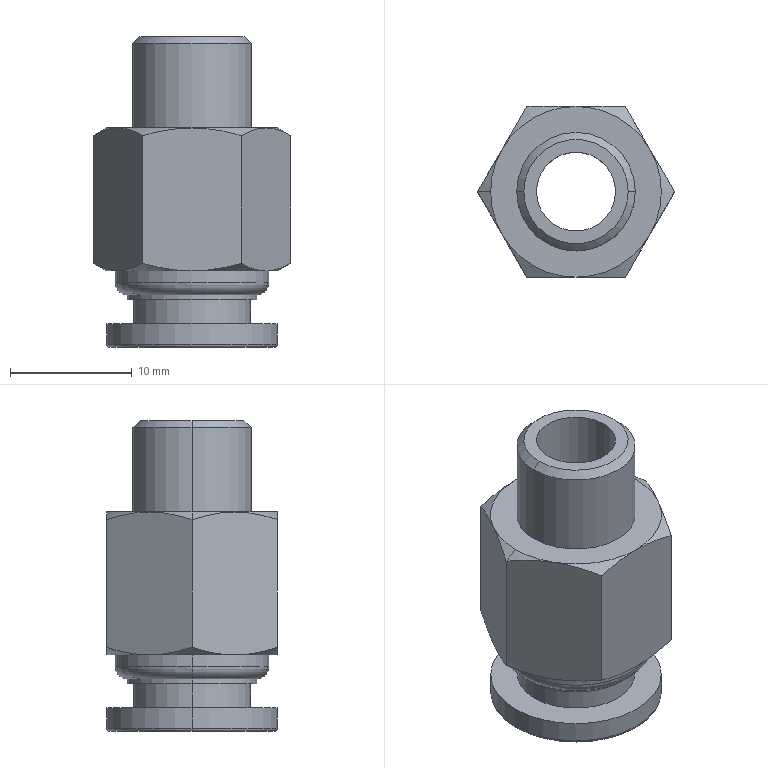Part | SolidWorks | features ICE 1, Revolution 1 | 1 solid | 47 faces | box 16.166 x 14 x 25.5 mm | volume 2115 mm3 | cone 16 | cylinder 14 | plane 13 | torus 4 | commonest cylinder face diameters 6.485 x2 8 x2 9.6 x2 9.728 x2 10.6 x2 12.6 x2
STEP:
#1=CARTESIAN_POINT('',(4.283,0.,25.5));
#2=VERTEX_POINT('',#1);
#3=CARTESIAN_POINT('',(-4.283,0.,25.5));
#4=VERTEX_POINT('',#3);
#5=CARTESIAN_POINT('',(0.,0.,25.5));
#6=DIRECTION('',(0.,0.,1.));
#7=DIRECTION('',(1.,0.,0.));
#8=AXIS2_PLACEMENT_3D('',#5,#6,#7);
#9=CIRCLE('',#8,4.283);
#10=EDGE_CURVE('',#2,#4,#9,.T.);
#11=ORIENTED_EDGE('',*,*,#10,.F.);
#12=CARTESIAN_POINT('',(4.864,0.,24.919));
#13=VERTEX_POINT('',#12);
#14=CARTESIAN_POINT('',(4.864,0.,24.919));
#15=DIRECTION('',(0.7071,0.,-0.7071));
#16=VECTOR('',#15,1000.);
#17=LINE('',#14,#16);
#18=EDGE_CURVE('',#2,#13,#17,.T.);
#19=ORIENTED_EDGE('',*,*,#18,.T.);
#20=CARTESIAN_POINT('',(-4.864,0.,24.919));
#21=VERTEX_POINT('',#20);
#22=CARTESIAN_POINT('',(0.,0.,24.919));
#23=DIRECTION('',(0.,0.,1.));
#24=DIRECTION('',(1.,0.,0.));
#25=AXIS2_PLACEMENT_3D('',#22,#23,#24);
#26=CIRCLE('',#25,4.864);
#27=EDGE_CURVE('',#13,#21,#26,.T.);
#28=ORIENTED_EDGE('',*,*,#27,.T.);
#29=CARTESIAN_POINT('',(-4.864,0.,24.919));
#30=DIRECTION('',(-0.7071,0.,-0.7071));
#31=VECTOR('',#30,1000.);
#32=LINE('',#29,#31);
#33=EDGE_CURVE('',#4,#21,#32,.T.);
#34=ORIENTED_EDGE('',*,*,#33,.F.);
#35=EDGE_LOOP('',(#11,#19,#28,#34));
#36=FACE_OUTER_BOUND('',#35,.T.);
#37=CARTESIAN_POINT('',(0.,0.,24.919));
#38=DIRECTION('',(0.,0.,-1.));
#39=DIRECTION('',(-1.,0.,0.));
#40=AXIS2_PLACEMENT_3D('',#37,#38,#39);
#41=CONICAL_SURFACE('',#40,4.864,0.7854);
#42=ADVANCED_FACE('',(#36),#41,.T.);
#43=CARTESIAN_POINT('',(4.864,0.,18.));
#44=VERTEX_POINT('',#43);
#45=CARTESIAN_POINT('',(-4.864,0.,18.));
#46=VERTEX_POINT('',#45);
#47=CARTESIAN_POINT('',(0.,0.,18.));
#48=DIRECTION('',(0.,0.,1.));
#49=DIRECTION('',(1.,0.,0.));
#50=AXIS2_PLACEMENT_3D('',#47,#48,#49);
#51=CIRCLE('',#50,4.864);
#52=EDGE_CURVE('',#44,#46,#51,.T.);
#53=ORIENTED_EDGE('',*,*,#52,.T.);
#54=CARTESIAN_POINT('',(-4.864,0.,0.));
#55=DIRECTION('',(0.,0.,1.));
#56=VECTOR('',#55,1000.);
#57=LINE('',#54,#56);
#58=EDGE_CURVE('',#46,#21,#57,.T.);
#59=ORIENTED_EDGE('',*,*,#58,.T.);
#60=ORIENTED_EDGE('',*,*,#27,.F.);
#61=CARTESIAN_POINT('',(4.864,0.,0.));
#62=DIRECTION('',(0.,0.,1.));
#63=VECTOR('',#62,1000.);
#64=LINE('',#61,#63);
#65=EDGE_CURVE('',#44,#13,#64,.T.);
#66=ORIENTED_EDGE('',*,*,#65,.F.);
#67=EDGE_LOOP('',(#53,#59,#60,#66));
#68=FACE_OUTER_BOUND('',#67,.T.);
#69=CARTESIAN_POINT('',(0.,0.,0.));
#70=DIRECTION('',(0.,0.,1.));
#71=DIRECTION('',(1.,0.,0.));
#72=AXIS2_PLACEMENT_3D('',#69,#70,#71);
#73=CYLINDRICAL_SURFACE('',#72,4.864);
#74=ADVANCED_FACE('',(#68),#73,.T.);
#75=CARTESIAN_POINT('',(6.3,0.,5.315));
#76=VERTEX_POINT('',#75);
#77=CARTESIAN_POINT('',(-6.3,0.,5.315));
#78=VERTEX_POINT('',#77);
#79=CARTESIAN_POINT('',(0.,0.,5.315));
#80=DIRECTION('',(0.,0.,1.));
#81=DIRECTION('',(1.,0.,0.));
#82=AXIS2_PLACEMENT_3D('',#79,#80,#81);
#83=CIRCLE('',#82,6.3);
#84=EDGE_CURVE('',#76,#78,#83,.T.);
#85=ORIENTED_EDGE('',*,*,#84,.T.);
#86=CARTESIAN_POINT('',(-6.3,0.,6.277));
#87=VERTEX_POINT('',#86);
#88=CARTESIAN_POINT('',(-6.3,0.,0.));
#89=DIRECTION('',(0.,0.,1.));
#90=VECTOR('',#89,1000.);
#91=LINE('',#88,#90);
#92=EDGE_CURVE('',#78,#87,#91,.T.);
#93=ORIENTED_EDGE('',*,*,#92,.T.);
#94=CARTESIAN_POINT('',(6.3,0.,6.277));
#95=VERTEX_POINT('',#94);
#96=CARTESIAN_POINT('',(0.,0.,6.277));
#97=DIRECTION('',(0.,0.,1.));
#98=DIRECTION('',(1.,0.,0.));
#99=AXIS2_PLACEMENT_3D('',#96,#97,#98);
#100=CIRCLE('',#99,6.3);
#101=EDGE_CURVE('',#95,#87,#100,.T.);
#102=ORIENTED_EDGE('',*,*,#101,.F.);
#103=CARTESIAN_POINT('',(6.3,0.,0.));
#104=DIRECTION('',(0.,0.,1.));
#105=VECTOR('',#104,1000.);
#106=LINE('',#103,#105);
#107=EDGE_CURVE('',#76,#95,#106,.T.);
#108=ORIENTED_EDGE('',*,*,#107,.F.);
#109=EDGE_LOOP('',(#85,#93,#102,#108));
#110=FACE_OUTER_BOUND('',#109,.T.);
#111=CARTESIAN_POINT('',(0.,0.,0.));
#112=DIRECTION('',(0.,0.,1.));
#113=DIRECTION('',(1.,0.,0.));
#114=AXIS2_PLACEMENT_3D('',#111,#112,#113);
#115=CYLINDRICAL_SURFACE('',#114,6.3);
#116=ADVANCED_FACE('',(#110),#115,.T.);
#117=CARTESIAN_POINT('',(5.3,0.,4.315));
#118=VERTEX_POINT('',#117);
#119=CARTESIAN_POINT('',(-5.3,0.,4.315));
#120=VERTEX_POINT('',#119);
#121=CARTESIAN_POINT('',(0.,0.,4.315));
#122=DIRECTION('',(0.,0.,1.));
#123=DIRECTION('',(1.,0.,0.));
#124=AXIS2_PLACEMENT_3D('',#121,#122,#123);
#125=CIRCLE('',#124,5.3);
#126=EDGE_CURVE('',#118,#120,#125,.T.);
#127=ORIENTED_EDGE('',*,*,#126,.T.);
#128=CARTESIAN_POINT('',(-5.3,0.,5.315));
#129=DIRECTION('',(0.,1.,0.));
#130=DIRECTION('',(-1.,0.,0.));
#131=AXIS2_PLACEMENT_3D('',#128,#129,#130);
#132=CIRCLE('',#131,1.);
#133=EDGE_CURVE('',#120,#78,#132,.T.);
#134=ORIENTED_EDGE('',*,*,#133,.T.);
#135=ORIENTED_EDGE('',*,*,#84,.F.);
#136=CARTESIAN_POINT('',(5.3,0.,5.315));
#137=DIRECTION('',(0.,-1.,0.));
#138=DIRECTION('',(0.,0.,-1.));
#139=AXIS2_PLACEMENT_3D('',#136,#137,#138);
#140=CIRCLE('',#139,1.);
#141=EDGE_CURVE('',#118,#76,#140,.T.);
#142=ORIENTED_EDGE('',*,*,#141,.F.);
#143=EDGE_LOOP('',(#127,#134,#135,#142));
#144=FACE_OUTER_BOUND('',#143,.T.);
#145=CARTESIAN_POINT('',(0.,0.,5.315));
#146=DIRECTION('',(0.,0.,1.));
#147=DIRECTION('',(1.,0.,0.));
#148=AXIS2_PLACEMENT_3D('',#145,#146,#147);
#149=TOROIDAL_SURFACE('',#148,5.3,1.);
#150=ADVANCED_FACE('',(#144),#149,.T.);
#151=CARTESIAN_POINT('',(5.3,0.,3.923));
#152=VERTEX_POINT('',#151);
#153=CARTESIAN_POINT('',(-5.3,0.,3.923));
#154=VERTEX_POINT('',#153);
#155=CARTESIAN_POINT('',(0.,0.,3.923));
#156=DIRECTION('',(0.,0.,1.));
#157=DIRECTION('',(1.,0.,0.));
#158=AXIS2_PLACEMENT_3D('',#155,#156,#157);
#159=CIRCLE('',#158,5.3);
#160=EDGE_CURVE('',#152,#154,#159,.T.);
#161=ORIENTED_EDGE('',*,*,#160,.T.);
#162=CARTESIAN_POINT('',(-5.3,0.,0.));
#163=DIRECTION('',(0.,0.,1.));
#164=VECTOR('',#163,1000.);
#165=LINE('',#162,#164);
#166=EDGE_CURVE('',#154,#120,#165,.T.);
#167=ORIENTED_EDGE('',*,*,#166,.T.);
#168=ORIENTED_EDGE('',*,*,#126,.F.);
#169=CARTESIAN_POINT('',(5.3,0.,0.));
#170=DIRECTION('',(0.,0.,1.));
#171=VECTOR('',#170,1000.);
#172=LINE('',#169,#171);
#173=EDGE_CURVE('',#152,#118,#172,.T.);
#174=ORIENTED_EDGE('',*,*,#173,.F.);
#175=EDGE_LOOP('',(#161,#167,#168,#174));
#176=FACE_OUTER_BOUND('',#175,.T.);
#177=CARTESIAN_POINT('',(0.,0.,0.));
#178=DIRECTION('',(0.,0.,1.));
#179=DIRECTION('',(1.,0.,0.));
#180=AXIS2_PLACEMENT_3D('',#177,#178,#179);
#181=CYLINDRICAL_SURFACE('',#180,5.3);
#182=ADVANCED_FACE('',(#176),#181,.T.);
#183=CARTESIAN_POINT('',(4.8,0.,1.962));
#184=VERTEX_POINT('',#183);
#185=CARTESIAN_POINT('',(-4.8,0.,1.962));
#186=VERTEX_POINT('',#185);
#187=CARTESIAN_POINT('',(0.,0.,1.962));
#188=DIRECTION('',(0.,0.,1.));
#189=DIRECTION('',(1.,0.,0.));
#190=AXIS2_PLACEMENT_3D('',#187,#188,#189);
#191=CIRCLE('',#190,4.8);
#192=EDGE_CURVE('',#184,#186,#191,.T.);
#193=ORIENTED_EDGE('',*,*,#192,.T.);
#194=CARTESIAN_POINT('',(-4.8,0.,3.923));
#195=VERTEX_POINT('',#194);
#196=CARTESIAN_POINT('',(-4.8,0.,0.));
#197=DIRECTION('',(0.,0.,1.));
#198=VECTOR('',#197,1000.);
#199=LINE('',#196,#198);
#200=EDGE_CURVE('',#186,#195,#199,.T.);
#201=ORIENTED_EDGE('',*,*,#200,.T.);
#202=CARTESIAN_POINT('',(4.8,0.,3.923));
#203=VERTEX_POINT('',#202);
#204=CARTESIAN_POINT('',(0.,0.,3.923));
#205=DIRECTION('',(0.,0.,1.));
#206=DIRECTION('',(1.,0.,0.));
#207=AXIS2_PLACEMENT_3D('',#204,#205,#206);
#208=CIRCLE('',#207,4.8);
#209=EDGE_CURVE('',#203,#195,#208,.T.);
#210=ORIENTED_EDGE('',*,*,#209,.F.);
#211=CARTESIAN_POINT('',(4.8,0.,0.));
#212=DIRECTION('',(0.,0.,1.));
#213=VECTOR('',#212,1000.);
#214=LINE('',#211,#213);
#215=EDGE_CURVE('',#184,#203,#214,.T.);
#216=ORIENTED_EDGE('',*,*,#215,.F.);
#217=EDGE_LOOP('',(#193,#201,#210,#216));
#218=FACE_OUTER_BOUND('',#217,.T.);
#219=CARTESIAN_POINT('',(0.,0.,0.));
#220=DIRECTION('',(0.,0.,1.));
#221=DIRECTION('',(1.,0.,0.));
#222=AXIS2_PLACEMENT_3D('',#219,#220,#221);
#223=CYLINDRICAL_SURFACE('',#222,4.8);
#224=ADVANCED_FACE('',(#218),#223,.T.);
#225=CARTESIAN_POINT('',(7.,0.,0.25));
#226=VERTEX_POINT('',#225);
#227=CARTESIAN_POINT('',(-7.,0.,0.25));
#228=VERTEX_POINT('',#227);
#229=CARTESIAN_POINT('',(0.,0.,0.25));
#230=DIRECTION('',(0.,0.,1.));
#231=DIRECTION('',(1.,0.,0.));
#232=AXIS2_PLACEMENT_3D('',#229,#230,#231);
#233=CIRCLE('',#232,7.);
#234=EDGE_CURVE('',#226,#228,#233,.T.);
#235=ORIENTED_EDGE('',*,*,#234,.T.);
#236=CARTESIAN_POINT('',(-7.,0.,1.962));
#237=VERTEX_POINT('',#236);
#238=CARTESIAN_POINT('',(-7.,0.,0.));
#239=DIRECTION('',(0.,0.,1.));
#240=VECTOR('',#239,1000.);
#241=LINE('',#238,#240);
#242=EDGE_CURVE('',#228,#237,#241,.T.);
#243=ORIENTED_EDGE('',*,*,#242,.T.);
#244=CARTESIAN_POINT('',(7.,0.,1.962));
#245=VERTEX_POINT('',#244);
#246=CARTESIAN_POINT('',(0.,0.,1.962));
#247=DIRECTION('',(0.,0.,1.));
#248=DIRECTION('',(1.,0.,0.));
#249=AXIS2_PLACEMENT_3D('',#246,#247,#248);
#250=CIRCLE('',#249,7.);
#251=EDGE_CURVE('',#245,#237,#250,.T.);
#252=ORIENTED_EDGE('',*,*,#251,.F.);
#253=CARTESIAN_POINT('',(7.,0.,0.));
#254=DIRECTION('',(0.,0.,1.));
#255=VECTOR('',#254,1000.);
#256=LINE('',#253,#255);
#257=EDGE_CURVE('',#226,#245,#256,.T.);
#258=ORIENTED_EDGE('',*,*,#257,.F.);
#259=EDGE_LOOP('',(#235,#243,#252,#258));
#260=FACE_OUTER_BOUND('',#259,.T.);
#261=CARTESIAN_POINT('',(0.,0.,0.));
#262=DIRECTION('',(0.,0.,1.));
#263=DIRECTION('',(1.,0.,0.));
#264=AXIS2_PLACEMENT_3D('',#261,#262,#263);
#265=CYLINDRICAL_SURFACE('',#264,7.);
#266=ADVANCED_FACE('',(#260),#265,.T.);
#267=CARTESIAN_POINT('',(6.75,0.,0.));
#268=VERTEX_POINT('',#267);
#269=CARTESIAN_POINT('',(-6.75,0.,0.));
#270=VERTEX_POINT('',#269);
#271=CARTESIAN_POINT('',(0.,0.,0.));
#272=DIRECTION('',(0.,0.,1.));
#273=DIRECTION('',(1.,0.,0.));
#274=AXIS2_PLACEMENT_3D('',#271,#272,#273);
#275=CIRCLE('',#274,6.75);
#276=EDGE_CURVE('',#268,#270,#275,.T.);
#277=ORIENTED_EDGE('',*,*,#276,.T.);
#278=CARTESIAN_POINT('',(-6.75,0.,0.25));
#279=DIRECTION('',(0.,1.,0.));
#280=DIRECTION('',(-1.,0.,0.));
#281=AXIS2_PLACEMENT_3D('',#278,#279,#280);
#282=CIRCLE('',#281,0.25);
#283=EDGE_CURVE('',#270,#228,#282,.T.);
#284=ORIENTED_EDGE('',*,*,#283,.T.);
#285=ORIENTED_EDGE('',*,*,#234,.F.);
#286=CARTESIAN_POINT('',(6.75,0.,0.25));
#287=DIRECTION('',(0.,-1.,0.));
#288=DIRECTION('',(0.,0.,-1.));
#289=AXIS2_PLACEMENT_3D('',#286,#287,#288);
#290=CIRCLE('',#289,0.25);
#291=EDGE_CURVE('',#268,#226,#290,.T.);
#292=ORIENTED_EDGE('',*,*,#291,.F.);
#293=EDGE_LOOP('',(#277,#284,#285,#292));
#294=FACE_OUTER_BOUND('',#293,.T.);
#295=CARTESIAN_POINT('',(0.,0.,0.25));
#296=DIRECTION('',(0.,0.,1.));
#297=DIRECTION('',(1.,0.,0.));
#298=AXIS2_PLACEMENT_3D('',#295,#296,#297);
#299=TOROIDAL_SURFACE('',#298,6.75,0.25);
#300=ADVANCED_FACE('',(#294),#299,.T.);
#301=CARTESIAN_POINT('',(-4.,0.,0.));
#302=VERTEX_POINT('',#301);
#303=CARTESIAN_POINT('',(4.,0.,0.));
#304=VERTEX_POINT('',#303);
#305=CARTESIAN_POINT('',(0.,0.,0.));
#306=DIRECTION('',(0.,0.,1.));
#307=DIRECTION('',(1.,0.,0.));
#308=AXIS2_PLACEMENT_3D('',#305,#306,#307);
#309=CIRCLE('',#308,4.);
#310=EDGE_CURVE('',#302,#304,#309,.T.);
#311=ORIENTED_EDGE('',*,*,#310,.F.);
#312=CARTESIAN_POINT('',(-4.,0.,17.));
#313=VERTEX_POINT('',#312);
#314=CARTESIAN_POINT('',(-4.,0.,0.));
#315=DIRECTION('',(0.,0.,1.));
#316=VECTOR('',#315,1000.);
#317=LINE('',#314,#316);
#318=EDGE_CURVE('',#302,#313,#317,.T.);
#319=ORIENTED_EDGE('',*,*,#318,.T.);
#320=CARTESIAN_POINT('',(4.,0.,17.));
#321=VERTEX_POINT('',#320);
#322=CARTESIAN_POINT('',(0.,0.,17.));
#323=DIRECTION('',(0.,0.,1.));
#324=DIRECTION('',(1.,0.,0.));
#325=AXIS2_PLACEMENT_3D('',#322,#323,#324);
#326=CIRCLE('',#325,4.);
#327=EDGE_CURVE('',#313,#321,#326,.T.);
#328=ORIENTED_EDGE('',*,*,#327,.T.);
#329=CARTESIAN_POINT('',(4.,0.,0.));
#330=DIRECTION('',(0.,0.,1.));
#331=VECTOR('',#330,1000.);
#332=LINE('',#329,#331);
#333=EDGE_CURVE('',#304,#321,#332,.T.);
#334=ORIENTED_EDGE('',*,*,#333,.F.);
#335=EDGE_LOOP('',(#311,#319,#328,#334));
#336=FACE_OUTER_BOUND('',#335,.T.);
#337=CARTESIAN_POINT('',(0.,0.,0.));
#338=DIRECTION('',(0.,0.,1.));
#339=DIRECTION('',(1.,0.,0.));
#340=AXIS2_PLACEMENT_3D('',#337,#338,#339);
#341=CYLINDRICAL_SURFACE('',#340,4.);
#342=ADVANCED_FACE('',(#336),#341,.F.);
#343=CARTESIAN_POINT('',(-3.243,0.,17.));
#344=VERTEX_POINT('',#343);
#345=CARTESIAN_POINT('',(3.243,0.,17.));
#346=VERTEX_POINT('',#345);
#347=CARTESIAN_POINT('',(0.,0.,17.));
#348=DIRECTION('',(0.,0.,1.));
#349=DIRECTION('',(1.,0.,0.));
#350=AXIS2_PLACEMENT_3D('',#347,#348,#349);
#351=CIRCLE('',#350,3.243);
#352=EDGE_CURVE('',#344,#346,#351,.T.);
#353=ORIENTED_EDGE('',*,*,#352,.F.);
#354=CARTESIAN_POINT('',(-3.243,0.,25.5));
#355=VERTEX_POINT('',#354);
#356=CARTESIAN_POINT('',(-3.243,0.,0.));
#357=DIRECTION('',(0.,0.,1.));
#358=VECTOR('',#357,1000.);
#359=LINE('',#356,#358);
#360=EDGE_CURVE('',#344,#355,#359,.T.);
#361=ORIENTED_EDGE('',*,*,#360,.T.);
#362=CARTESIAN_POINT('',(3.243,0.,25.5));
#363=VERTEX_POINT('',#362);
#364=CARTESIAN_POINT('',(0.,0.,25.5));
#365=DIRECTION('',(0.,0.,1.));
#366=DIRECTION('',(1.,0.,0.));
#367=AXIS2_PLACEMENT_3D('',#364,#365,#366);
#368=CIRCLE('',#367,3.243);
#369=EDGE_CURVE('',#355,#363,#368,.T.);
#370=ORIENTED_EDGE('',*,*,#369,.T.);
#371=CARTESIAN_POINT('',(3.243,0.,0.));
#372=DIRECTION('',(0.,0.,1.));
#373=VECTOR('',#372,1000.);
#374=LINE('',#371,#373);
#375=EDGE_CURVE('',#346,#363,#374,.T.);
#376=ORIENTED_EDGE('',*,*,#375,.F.);
#377=EDGE_LOOP('',(#353,#361,#370,#376));
#378=FACE_OUTER_BOUND('',#377,.T.);
#379=CARTESIAN_POINT('',(0.,0.,0.));
#380=DIRECTION('',(0.,0.,1.));
#381=DIRECTION('',(1.,0.,0.));
#382=AXIS2_PLACEMENT_3D('',#379,#380,#381);
#383=CYLINDRICAL_SURFACE('',#382,3.243);
#384=ADVANCED_FACE('',(#378),#383,.F.);
#385=CARTESIAN_POINT('',(-7.,0.,18.));
#386=VERTEX_POINT('',#385);
#387=CARTESIAN_POINT('',(-6.062,-3.5,18.));
#388=VERTEX_POINT('',#387);
#389=CARTESIAN_POINT('',(0.,0.,18.));
#390=DIRECTION('',(0.,0.,1.));
#391=DIRECTION('',(1.,0.,0.));
#392=AXIS2_PLACEMENT_3D('',#389,#390,#391);
#393=CIRCLE('',#392,7.);
#394=EDGE_CURVE('',#386,#388,#393,.T.);
#395=ORIENTED_EDGE('',*,*,#394,.F.);
#396=CARTESIAN_POINT('',(-8.083,0.,17.375));
#397=VERTEX_POINT('',#396);
#398=CARTESIAN_POINT('',(-8.083,0.,17.375));
#399=DIRECTION('',(-0.866,0.,-0.5));
#400=VECTOR('',#399,1000.);
#401=LINE('',#398,#400);
#402=EDGE_CURVE('',#386,#397,#401,.T.);
#403=ORIENTED_EDGE('',*,*,#402,.T.);
#404=CARTESIAN_POINT('',(-6.062,-3.5,18.));
#405=CARTESIAN_POINT('',(-6.234,-3.203,18.));
#406=CARTESIAN_POINT('',(-6.406,-2.905,17.985));
#407=CARTESIAN_POINT('',(-6.747,-2.314,17.928));
#408=CARTESIAN_POINT('',(-6.916,-2.021,17.886));
#409=CARTESIAN_POINT('',(-7.421,-1.147,17.722));
#410=CARTESIAN_POINT('',(-7.753,-0.5711,17.565));
#411=CARTESIAN_POINT('',(-8.083,0.,17.375));
#412=B_SPLINE_CURVE_WITH_KNOTS('',3,(#404,#405,#406,#407,#408,#409,#410,#411),.UNSPECIFIED.,.F.,.F.,(4,2,2,4),(0.00409,0.005108,0.006127,0.008164),.UNSPECIFIED.);
#413=EDGE_CURVE('',#388,#397,#412,.T.);
#414=ORIENTED_EDGE('',*,*,#413,.F.);
#415=EDGE_LOOP('',(#395,#403,#414));
#416=FACE_OUTER_BOUND('',#415,.T.);
#417=CARTESIAN_POINT('',(0.,0.,17.375));
#418=DIRECTION('',(0.,0.,-1.));
#419=DIRECTION('',(-1.,0.,0.));
#420=AXIS2_PLACEMENT_3D('',#417,#418,#419);
#421=CONICAL_SURFACE('',#420,8.083,1.047);
#422=ADVANCED_FACE('',(#416),#421,.T.);
#423=CARTESIAN_POINT('',(6.062,-3.5,6.277));
#424=VERTEX_POINT('',#423);
#425=CARTESIAN_POINT('',(7.,0.,6.277));
#426=VERTEX_POINT('',#425);
#427=CARTESIAN_POINT('',(0.,0.,6.277));
#428=DIRECTION('',(0.,0.,1.));
#429=DIRECTION('',(1.,0.,0.));
#430=AXIS2_PLACEMENT_3D('',#427,#428,#429);
#431=CIRCLE('',#430,7.);
#432=EDGE_CURVE('',#424,#426,#431,.T.);
#433=ORIENTED_EDGE('',*,*,#432,.T.);
#434=CARTESIAN_POINT('',(8.083,0.,6.902));
#435=VERTEX_POINT('',#434);
#436=CARTESIAN_POINT('',(7.,0.,6.277));
#437=DIRECTION('',(0.866,0.,0.5));
#438=VECTOR('',#437,1000.);
#439=LINE('',#436,#438);
#440=EDGE_CURVE('',#426,#435,#439,.T.);
#441=ORIENTED_EDGE('',*,*,#440,.T.);
#442=CARTESIAN_POINT('',(6.062,-3.5,6.277));
#443=CARTESIAN_POINT('',(6.234,-3.203,6.277));
#444=CARTESIAN_POINT('',(6.406,-2.905,6.292));
#445=CARTESIAN_POINT('',(6.747,-2.314,6.349));
#446=CARTESIAN_POINT('',(6.916,-2.021,6.391));
#447=CARTESIAN_POINT('',(7.421,-1.147,6.555));
#448=CARTESIAN_POINT('',(7.753,-0.5711,6.712));
#449=CARTESIAN_POINT('',(8.083,0.,6.902));
#450=B_SPLINE_CURVE_WITH_KNOTS('',3,(#442,#443,#444,#445,#446,#447,#448,#449),.UNSPECIFIED.,.F.,.F.,(4,2,2,4),(0.00409,0.005108,0.006127,0.008164),.UNSPECIFIED.);
#451=EDGE_CURVE('',#424,#435,#450,.T.);
#452=ORIENTED_EDGE('',*,*,#451,.F.);
#453=EDGE_LOOP('',(#433,#441,#452));
#454=FACE_OUTER_BOUND('',#453,.T.);
#455=CARTESIAN_POINT('',(0.,0.,6.277));
#456=DIRECTION('',(0.,0.,1.));
#457=DIRECTION('',(1.,0.,0.));
#458=AXIS2_PLACEMENT_3D('',#455,#456,#457);
#459=CONICAL_SURFACE('',#458,7.,1.047);
#460=ADVANCED_FACE('',(#454),#459,.T.);
#461=CARTESIAN_POINT('',(4.041,-7.,6.902));
#462=VERTEX_POINT('',#461);
#463=CARTESIAN_POINT('',(4.041,-7.,6.902));
#464=CARTESIAN_POINT('',(4.372,-6.427,6.711));
#465=CARTESIAN_POINT('',(4.705,-5.851,6.554));
#466=CARTESIAN_POINT('',(5.378,-4.685,6.337));
#467=CARTESIAN_POINT('',(5.718,-4.096,6.277));
#468=CARTESIAN_POINT('',(6.062,-3.5,6.277));
#469=B_SPLINE_CURVE_WITH_KNOTS('',3,(#463,#464,#465,#466,#467,#468),.UNSPECIFIED.,.F.,.F.,(4,2,4),(0.000000238,0.002045,0.00409),.UNSPECIFIED.);
#470=EDGE_CURVE('',#462,#424,#469,.T.);
#471=ORIENTED_EDGE('',*,*,#470,.F.);
#472=CARTESIAN_POINT('',(0.,-7.,6.277));
#473=VERTEX_POINT('',#472);
#474=CARTESIAN_POINT('',(0.,-7.,6.277));
#475=CARTESIAN_POINT('',(0.6833,-7.,6.277));
#476=CARTESIAN_POINT('',(1.376,-7.,6.337));
#477=CARTESIAN_POINT('',(2.726,-7.,6.556));
#478=CARTESIAN_POINT('',(3.388,-7.,6.713));
#479=CARTESIAN_POINT('',(4.041,-7.,6.902));
#480=B_SPLINE_CURVE_WITH_KNOTS('',3,(#474,#475,#476,#477,#478,#479),.UNSPECIFIED.,.F.,.F.,(4,2,4),(0.0113,0.01334,0.01539),.UNSPECIFIED.);
#481=EDGE_CURVE('',#473,#462,#480,.T.);
#482=ORIENTED_EDGE('',*,*,#481,.F.);
#483=CARTESIAN_POINT('',(0.,0.,6.277));
#484=DIRECTION('',(0.,0.,1.));
#485=DIRECTION('',(1.,0.,0.));
#486=AXIS2_PLACEMENT_3D('',#483,#484,#485);
#487=CIRCLE('',#486,7.);
#488=EDGE_CURVE('',#473,#424,#487,.T.);
#489=ORIENTED_EDGE('',*,*,#488,.T.);
#490=EDGE_LOOP('',(#471,#482,#489));
#491=FACE_OUTER_BOUND('',#490,.T.);
#492=CARTESIAN_POINT('',(0.,0.,6.277));
#493=DIRECTION('',(0.,0.,1.));
#494=DIRECTION('',(1.,0.,0.));
#495=AXIS2_PLACEMENT_3D('',#492,#493,#494);
#496=CONICAL_SURFACE('',#495,7.,1.047);
#497=ADVANCED_FACE('',(#491),#496,.T.);
#498=ORIENTED_EDGE('',*,*,#440,.F.);
#499=CARTESIAN_POINT('',(6.062,3.5,6.277));
#500=VERTEX_POINT('',#499);
#501=CARTESIAN_POINT('',(0.,0.,6.277));
#502=DIRECTION('',(0.,0.,1.));
#503=DIRECTION('',(1.,0.,0.));
#504=AXIS2_PLACEMENT_3D('',#501,#502,#503);
#505=CIRCLE('',#504,7.);
#506=EDGE_CURVE('',#426,#500,#505,.T.);
#507=ORIENTED_EDGE('',*,*,#506,.T.);
#508=CARTESIAN_POINT('',(8.083,0.,6.902));
#509=CARTESIAN_POINT('',(7.752,0.5726,6.711));
#510=CARTESIAN_POINT('',(7.419,1.149,6.554));
#511=CARTESIAN_POINT('',(6.746,2.315,6.337));
#512=CARTESIAN_POINT('',(6.406,2.904,6.277));
#513=CARTESIAN_POINT('',(6.062,3.5,6.277));
#514=B_SPLINE_CURVE_WITH_KNOTS('',3,(#508,#509,#510,#511,#512,#513),.UNSPECIFIED.,.F.,.F.,(4,2,4),(0.000000238,0.002045,0.00409),.UNSPECIFIED.);
#515=EDGE_CURVE('',#435,#500,#514,.T.);
#516=ORIENTED_EDGE('',*,*,#515,.F.);
#517=EDGE_LOOP('',(#498,#507,#516));
#518=FACE_OUTER_BOUND('',#517,.T.);
#519=CARTESIAN_POINT('',(0.,0.,6.277));
#520=DIRECTION('',(0.,0.,1.));
#521=DIRECTION('',(1.,0.,0.));
#522=AXIS2_PLACEMENT_3D('',#519,#520,#521);
#523=CONICAL_SURFACE('',#522,7.,1.047);
#524=ADVANCED_FACE('',(#518),#523,.T.);
#525=CARTESIAN_POINT('',(4.041,7.,6.902));
#526=VERTEX_POINT('',#525);
#527=CARTESIAN_POINT('',(6.062,3.5,6.277));
#528=CARTESIAN_POINT('',(5.891,3.797,6.277));
#529=CARTESIAN_POINT('',(5.718,4.095,6.292));
#530=CARTESIAN_POINT('',(5.378,4.686,6.349));
#531=CARTESIAN_POINT('',(5.208,4.979,6.391));
#532=CARTESIAN_POINT('',(4.704,5.853,6.555));
#533=CARTESIAN_POINT('',(4.371,6.429,6.712));
#534=CARTESIAN_POINT('',(4.041,7.,6.902));
#535=B_SPLINE_CURVE_WITH_KNOTS('',3,(#527,#528,#529,#530,#531,#532,#533,#534),.UNSPECIFIED.,.F.,.F.,(4,2,2,4),(0.00409,0.005108,0.006127,0.008164),.UNSPECIFIED.);
#536=EDGE_CURVE('',#500,#526,#535,.T.);
#537=ORIENTED_EDGE('',*,*,#536,.F.);
#538=CARTESIAN_POINT('',(0.,7.,6.277));
#539=VERTEX_POINT('',#538);
#540=CARTESIAN_POINT('',(0.,0.,6.277));
#541=DIRECTION('',(0.,0.,1.));
#542=DIRECTION('',(1.,0.,0.));
#543=AXIS2_PLACEMENT_3D('',#540,#541,#542);
#544=CIRCLE('',#543,7.);
#545=EDGE_CURVE('',#500,#539,#544,.T.);
#546=ORIENTED_EDGE('',*,*,#545,.T.);
#547=CARTESIAN_POINT('',(4.041,7.,6.902));
#548=CARTESIAN_POINT('',(3.388,7.,6.713));
#549=CARTESIAN_POINT('',(2.726,7.,6.556));
#550=CARTESIAN_POINT('',(1.376,7.,6.337));
#551=CARTESIAN_POINT('',(0.6833,7.,6.277));
#552=CARTESIAN_POINT('',(0.,7.,6.277));
#553=B_SPLINE_CURVE_WITH_KNOTS('',3,(#547,#548,#549,#550,#551,#552),.UNSPECIFIED.,.F.,.F.,(4,2,4),(0.002962,0.005003,0.007043),.UNSPECIFIED.);
#554=EDGE_CURVE('',#526,#539,#553,.T.);
#555=ORIENTED_EDGE('',*,*,#554,.F.);
#556=EDGE_LOOP('',(#537,#546,#555));
#557=FACE_OUTER_BOUND('',#556,.T.);
#558=CARTESIAN_POINT('',(0.,0.,6.277));
#559=DIRECTION('',(0.,0.,1.));
#560=DIRECTION('',(1.,0.,0.));
#561=AXIS2_PLACEMENT_3D('',#558,#559,#560);
#562=CONICAL_SURFACE('',#561,7.,1.047);
#563=ADVANCED_FACE('',(#557),#562,.T.);
#564=CARTESIAN_POINT('',(-4.041,7.,6.902));
#565=VERTEX_POINT('',#564);
#566=CARTESIAN_POINT('',(0.,7.,6.277));
#567=CARTESIAN_POINT('',(-0.6829,7.,6.277));
#568=CARTESIAN_POINT('',(-1.361,7.,6.336));
#569=CARTESIAN_POINT('',(-2.711,7.,6.553));
#570=CARTESIAN_POINT('',(-3.384,7.,6.712));
#571=CARTESIAN_POINT('',(-4.041,7.,6.902));
#572=B_SPLINE_CURVE_WITH_KNOTS('',3,(#566,#567,#568,#569,#570,#571),.UNSPECIFIED.,.F.,.F.,(4,2,4),(0.007043,0.009082,0.01112),.UNSPECIFIED.);
#573=EDGE_CURVE('',#539,#565,#572,.T.);
#574=ORIENTED_EDGE('',*,*,#573,.F.);
#575=CARTESIAN_POINT('',(-6.062,3.5,6.277));
#576=VERTEX_POINT('',#575);
#577=CARTESIAN_POINT('',(0.,0.,6.277));
#578=DIRECTION('',(0.,0.,1.));
#579=DIRECTION('',(1.,0.,0.));
#580=AXIS2_PLACEMENT_3D('',#577,#578,#579);
#581=CIRCLE('',#580,7.);
#582=EDGE_CURVE('',#539,#576,#581,.T.);
#583=ORIENTED_EDGE('',*,*,#582,.T.);
#584=CARTESIAN_POINT('',(-4.041,7.,6.902));
#585=CARTESIAN_POINT('',(-4.372,6.427,6.711));
#586=CARTESIAN_POINT('',(-4.705,5.851,6.554));
#587=CARTESIAN_POINT('',(-5.378,4.685,6.337));
#588=CARTESIAN_POINT('',(-5.718,4.096,6.277));
#589=CARTESIAN_POINT('',(-6.062,3.5,6.277));
#590=B_SPLINE_CURVE_WITH_KNOTS('',3,(#584,#585,#586,#587,#588,#589),.UNSPECIFIED.,.F.,.F.,(4,2,4),(0.000000238,0.002045,0.00409),.UNSPECIFIED.);
#591=EDGE_CURVE('',#565,#576,#590,.T.);
#592=ORIENTED_EDGE('',*,*,#591,.F.);
#593=EDGE_LOOP('',(#574,#583,#592));
#594=FACE_OUTER_BOUND('',#593,.T.);
#595=CARTESIAN_POINT('',(0.,0.,6.277));
#596=DIRECTION('',(0.,0.,1.));
#597=DIRECTION('',(1.,0.,0.));
#598=AXIS2_PLACEMENT_3D('',#595,#596,#597);
#599=CONICAL_SURFACE('',#598,7.,1.047);
#600=ADVANCED_FACE('',(#594),#599,.T.);
#601=CARTESIAN_POINT('',(-8.083,0.,6.902));
#602=VERTEX_POINT('',#601);
#603=CARTESIAN_POINT('',(-6.062,3.5,6.277));
#604=CARTESIAN_POINT('',(-6.234,3.203,6.277));
#605=CARTESIAN_POINT('',(-6.406,2.905,6.292));
#606=CARTESIAN_POINT('',(-6.747,2.314,6.349));
#607=CARTESIAN_POINT('',(-6.916,2.021,6.391));
#608=CARTESIAN_POINT('',(-7.421,1.147,6.555));
#609=CARTESIAN_POINT('',(-7.753,0.5711,6.712));
#610=CARTESIAN_POINT('',(-8.083,0.,6.902));
#611=B_SPLINE_CURVE_WITH_KNOTS('',3,(#603,#604,#605,#606,#607,#608,#609,#610),.UNSPECIFIED.,.F.,.F.,(4,2,2,4),(0.00409,0.005108,0.006127,0.008164),.UNSPECIFIED.);
#612=EDGE_CURVE('',#576,#602,#611,.T.);
#613=ORIENTED_EDGE('',*,*,#612,.F.);
#614=CARTESIAN_POINT('',(-6.062,-3.5,6.277));
#615=VERTEX_POINT('',#614);
#616=CARTESIAN_POINT('',(0.,0.,6.277));
#617=DIRECTION('',(0.,0.,1.));
#618=DIRECTION('',(1.,0.,0.));
#619=AXIS2_PLACEMENT_3D('',#616,#617,#618);
#620=CIRCLE('',#619,7.);
#621=EDGE_CURVE('',#576,#615,#620,.T.);
#622=ORIENTED_EDGE('',*,*,#621,.T.);
#623=CARTESIAN_POINT('',(-8.083,0.,6.902));
#624=CARTESIAN_POINT('',(-7.752,-0.5726,6.711));
#625=CARTESIAN_POINT('',(-7.419,-1.149,6.554));
#626=CARTESIAN_POINT('',(-6.746,-2.315,6.337));
#627=CARTESIAN_POINT('',(-6.406,-2.904,6.277));
#628=CARTESIAN_POINT('',(-6.062,-3.5,6.277));
#629=B_SPLINE_CURVE_WITH_KNOTS('',3,(#623,#624,#625,#626,#627,#628),.UNSPECIFIED.,.F.,.F.,(4,2,4),(0.000000238,0.002045,0.00409),.UNSPECIFIED.);
#630=EDGE_CURVE('',#602,#615,#629,.T.);
#631=ORIENTED_EDGE('',*,*,#630,.F.);
#632=EDGE_LOOP('',(#613,#622,#631));
#633=FACE_OUTER_BOUND('',#632,.T.);
#634=CARTESIAN_POINT('',(0.,0.,6.277));
#635=DIRECTION('',(0.,0.,1.));
#636=DIRECTION('',(1.,0.,0.));
#637=AXIS2_PLACEMENT_3D('',#634,#635,#636);
#638=CONICAL_SURFACE('',#637,7.,1.047);
#639=ADVANCED_FACE('',(#633),#638,.T.);
#640=CARTESIAN_POINT('',(-4.041,-7.,6.902));
#641=VERTEX_POINT('',#640);
#642=CARTESIAN_POINT('',(-6.062,-3.5,6.277));
#643=CARTESIAN_POINT('',(-5.891,-3.797,6.277));
#644=CARTESIAN_POINT('',(-5.718,-4.095,6.292));
#645=CARTESIAN_POINT('',(-5.378,-4.686,6.349));
#646=CARTESIAN_POINT('',(-5.208,-4.979,6.391));
#647=CARTESIAN_POINT('',(-4.704,-5.853,6.555));
#648=CARTESIAN_POINT('',(-4.371,-6.429,6.712));
#649=CARTESIAN_POINT('',(-4.041,-7.,6.902));
#650=B_SPLINE_CURVE_WITH_KNOTS('',3,(#642,#643,#644,#645,#646,#647,#648,#649),.UNSPECIFIED.,.F.,.F.,(4,2,2,4),(0.00409,0.005108,0.006127,0.008164),.UNSPECIFIED.);
#651=EDGE_CURVE('',#615,#641,#650,.T.);
#652=ORIENTED_EDGE('',*,*,#651,.F.);
#653=CARTESIAN_POINT('',(0.,0.,6.277));
#654=DIRECTION('',(0.,0.,1.));
#655=DIRECTION('',(1.,0.,0.));
#656=AXIS2_PLACEMENT_3D('',#653,#654,#655);
#657=CIRCLE('',#656,7.);
#658=EDGE_CURVE('',#615,#473,#657,.T.);
#659=ORIENTED_EDGE('',*,*,#658,.T.);
#660=CARTESIAN_POINT('',(-4.041,-7.,6.902));
#661=CARTESIAN_POINT('',(-3.384,-7.,6.712));
#662=CARTESIAN_POINT('',(-2.711,-7.,6.553));
#663=CARTESIAN_POINT('',(-1.361,-7.,6.336));
#664=CARTESIAN_POINT('',(-0.6829,-7.,6.277));
#665=CARTESIAN_POINT('',(0.,-7.,6.277));
#666=B_SPLINE_CURVE_WITH_KNOTS('',3,(#660,#661,#662,#663,#664,#665),.UNSPECIFIED.,.F.,.F.,(4,2,4),(0.00721,0.009255,0.0113),.UNSPECIFIED.);
#667=EDGE_CURVE('',#641,#473,#666,.T.);
#668=ORIENTED_EDGE('',*,*,#667,.F.);
#669=EDGE_LOOP('',(#652,#659,#668));
#670=FACE_OUTER_BOUND('',#669,.T.);
#671=CARTESIAN_POINT('',(0.,0.,6.277));
#672=DIRECTION('',(0.,0.,1.));
#673=DIRECTION('',(1.,0.,0.));
#674=AXIS2_PLACEMENT_3D('',#671,#672,#673);
#675=CONICAL_SURFACE('',#674,7.,1.047);
#676=ADVANCED_FACE('',(#670),#675,.T.);
#677=CARTESIAN_POINT('',(-4.041,7.,17.375));
#678=VERTEX_POINT('',#677);
#679=CARTESIAN_POINT('',(0.,7.,18.));
#680=VERTEX_POINT('',#679);
#681=CARTESIAN_POINT('',(-4.041,7.,17.375));
#682=CARTESIAN_POINT('',(-3.384,7.,17.565));
#683=CARTESIAN_POINT('',(-2.711,7.,17.724));
#684=CARTESIAN_POINT('',(-1.361,7.,17.941));
#685=CARTESIAN_POINT('',(-0.6829,7.,18.));
#686=CARTESIAN_POINT('',(0.,7.,18.));
#687=B_SPLINE_CURVE_WITH_KNOTS('',3,(#681,#682,#683,#684,#685,#686),.UNSPECIFIED.,.F.,.F.,(4,2,4),(0.00721,0.009255,0.0113),.UNSPECIFIED.);
#688=EDGE_CURVE('',#678,#680,#687,.T.);
#689=ORIENTED_EDGE('',*,*,#688,.F.);
#690=CARTESIAN_POINT('',(-6.062,3.5,18.));
#691=VERTEX_POINT('',#690);
#692=CARTESIAN_POINT('',(-6.062,3.5,18.));
#693=CARTESIAN_POINT('',(-5.891,3.797,18.));
#694=CARTESIAN_POINT('',(-5.718,4.095,17.985));
#695=CARTESIAN_POINT('',(-5.378,4.686,17.928));
#696=CARTESIAN_POINT('',(-5.208,4.979,17.886));
#697=CARTESIAN_POINT('',(-4.704,5.853,17.722));
#698=CARTESIAN_POINT('',(-4.371,6.429,17.565));
#699=CARTESIAN_POINT('',(-4.041,7.,17.375));
#700=B_SPLINE_CURVE_WITH_KNOTS('',3,(#692,#693,#694,#695,#696,#697,#698,#699),.UNSPECIFIED.,.F.,.F.,(4,2,2,4),(0.00409,0.005108,0.006127,0.008164),.UNSPECIFIED.);
#701=EDGE_CURVE('',#691,#678,#700,.T.);
#702=ORIENTED_EDGE('',*,*,#701,.F.);
#703=CARTESIAN_POINT('',(0.,0.,18.));
#704=DIRECTION('',(0.,0.,1.));
#705=DIRECTION('',(1.,0.,0.));
#706=AXIS2_PLACEMENT_3D('',#703,#704,#705);
#707=CIRCLE('',#706,7.);
#708=EDGE_CURVE('',#680,#691,#707,.T.);
#709=ORIENTED_EDGE('',*,*,#708,.F.);
#710=EDGE_LOOP('',(#689,#702,#709));
#711=FACE_OUTER_BOUND('',#710,.T.);
#712=CARTESIAN_POINT('',(0.,0.,17.375));
#713=DIRECTION('',(0.,0.,-1.));
#714=DIRECTION('',(-1.,0.,0.));
#715=AXIS2_PLACEMENT_3D('',#712,#713,#714);
#716=CONICAL_SURFACE('',#715,8.083,1.047);
#717=ADVANCED_FACE('',(#711),#716,.T.);
#718=CARTESIAN_POINT('',(4.041,7.,17.375));
#719=VERTEX_POINT('',#718);
#720=CARTESIAN_POINT('',(0.,7.,18.));
#721=CARTESIAN_POINT('',(0.6833,7.,18.));
#722=CARTESIAN_POINT('',(1.376,7.,17.94));
#723=CARTESIAN_POINT('',(2.726,7.,17.721));
#724=CARTESIAN_POINT('',(3.388,7.,17.563));
#725=CARTESIAN_POINT('',(4.041,7.,17.375));
#726=B_SPLINE_CURVE_WITH_KNOTS('',3,(#720,#721,#722,#723,#724,#725),.UNSPECIFIED.,.F.,.F.,(4,2,4),(0.0113,0.01334,0.01539),.UNSPECIFIED.);
#727=EDGE_CURVE('',#680,#719,#726,.T.);
#728=ORIENTED_EDGE('',*,*,#727,.F.);
#729=CARTESIAN_POINT('',(6.062,3.5,18.));
#730=VERTEX_POINT('',#729);
#731=CARTESIAN_POINT('',(0.,0.,18.));
#732=DIRECTION('',(0.,0.,1.));
#733=DIRECTION('',(1.,0.,0.));
#734=AXIS2_PLACEMENT_3D('',#731,#732,#733);
#735=CIRCLE('',#734,7.);
#736=EDGE_CURVE('',#730,#680,#735,.T.);
#737=ORIENTED_EDGE('',*,*,#736,.F.);
#738=CARTESIAN_POINT('',(4.041,7.,17.375));
#739=CARTESIAN_POINT('',(4.372,6.427,17.566));
#740=CARTESIAN_POINT('',(4.705,5.851,17.723));
#741=CARTESIAN_POINT('',(5.378,4.685,17.94));
#742=CARTESIAN_POINT('',(5.718,4.096,18.));
#743=CARTESIAN_POINT('',(6.062,3.5,18.));
#744=B_SPLINE_CURVE_WITH_KNOTS('',3,(#738,#739,#740,#741,#742,#743),.UNSPECIFIED.,.F.,.F.,(4,2,4),(0.000000238,0.002045,0.00409),.UNSPECIFIED.);
#745=EDGE_CURVE('',#719,#730,#744,.T.);
#746=ORIENTED_EDGE('',*,*,#745,.F.);
#747=EDGE_LOOP('',(#728,#737,#746));
#748=FACE_OUTER_BOUND('',#747,.T.);
#749=CARTESIAN_POINT('',(0.,0.,17.375));
#750=DIRECTION('',(0.,0.,-1.));
#751=DIRECTION('',(-1.,0.,0.));
#752=AXIS2_PLACEMENT_3D('',#749,#750,#751);
#753=CONICAL_SURFACE('',#752,8.083,1.047);
#754=ADVANCED_FACE('',(#748),#753,.T.);
#755=CARTESIAN_POINT('',(8.083,0.,17.375));
#756=VERTEX_POINT('',#755);
#757=CARTESIAN_POINT('',(6.062,3.5,18.));
#758=CARTESIAN_POINT('',(6.234,3.203,18.));
#759=CARTESIAN_POINT('',(6.406,2.905,17.985));
#760=CARTESIAN_POINT('',(6.747,2.314,17.928));
#761=CARTESIAN_POINT('',(6.916,2.021,17.886));
#762=CARTESIAN_POINT('',(7.421,1.147,17.722));
#763=CARTESIAN_POINT('',(7.753,0.5711,17.565));
#764=CARTESIAN_POINT('',(8.083,0.,17.375));
#765=B_SPLINE_CURVE_WITH_KNOTS('',3,(#757,#758,#759,#760,#761,#762,#763,#764),.UNSPECIFIED.,.F.,.F.,(4,2,2,4),(0.00409,0.005108,0.006127,0.008164),.UNSPECIFIED.);
#766=EDGE_CURVE('',#730,#756,#765,.T.);
#767=ORIENTED_EDGE('',*,*,#766,.F.);
#768=CARTESIAN_POINT('',(6.062,-3.5,18.));
#769=VERTEX_POINT('',#768);
#770=CARTESIAN_POINT('',(0.,0.,18.));
#771=DIRECTION('',(0.,0.,1.));
#772=DIRECTION('',(1.,0.,0.));
#773=AXIS2_PLACEMENT_3D('',#770,#771,#772);
#774=CIRCLE('',#773,7.);
#775=EDGE_CURVE('',#769,#730,#774,.T.);
#776=ORIENTED_EDGE('',*,*,#775,.F.);
#777=CARTESIAN_POINT('',(8.083,0.,17.375));
#778=CARTESIAN_POINT('',(7.752,-0.5726,17.566));
#779=CARTESIAN_POINT('',(7.419,-1.149,17.723));
#780=CARTESIAN_POINT('',(6.746,-2.315,17.94));
#781=CARTESIAN_POINT('',(6.406,-2.904,18.));
#782=CARTESIAN_POINT('',(6.062,-3.5,18.));
#783=B_SPLINE_CURVE_WITH_KNOTS('',3,(#777,#778,#779,#780,#781,#782),.UNSPECIFIED.,.F.,.F.,(4,2,4),(0.000000238,0.002045,0.00409),.UNSPECIFIED.);
#784=EDGE_CURVE('',#756,#769,#783,.T.);
#785=ORIENTED_EDGE('',*,*,#784,.F.);
#786=EDGE_LOOP('',(#767,#776,#785));
#787=FACE_OUTER_BOUND('',#786,.T.);
#788=CARTESIAN_POINT('',(0.,0.,17.375));
#789=DIRECTION('',(0.,0.,-1.));
#790=DIRECTION('',(-1.,0.,0.));
#791=AXIS2_PLACEMENT_3D('',#788,#789,#790);
#792=CONICAL_SURFACE('',#791,8.083,1.047);
#793=ADVANCED_FACE('',(#787),#792,.T.);
#794=ORIENTED_EDGE('',*,*,#402,.F.);
#795=CARTESIAN_POINT('',(0.,0.,18.));
#796=DIRECTION('',(0.,0.,1.));
#797=DIRECTION('',(1.,0.,0.));
#798=AXIS2_PLACEMENT_3D('',#795,#796,#797);
#799=CIRCLE('',#798,7.);
#800=EDGE_CURVE('',#691,#386,#799,.T.);
#801=ORIENTED_EDGE('',*,*,#800,.F.);
#802=CARTESIAN_POINT('',(-8.083,0.,17.375));
#803=CARTESIAN_POINT('',(-7.752,0.5726,17.566));
#804=CARTESIAN_POINT('',(-7.419,1.149,17.723));
#805=CARTESIAN_POINT('',(-6.746,2.315,17.94));
#806=CARTESIAN_POINT('',(-6.406,2.904,18.));
#807=CARTESIAN_POINT('',(-6.062,3.5,18.));
#808=B_SPLINE_CURVE_WITH_KNOTS('',3,(#802,#803,#804,#805,#806,#807),.UNSPECIFIED.,.F.,.F.,(4,2,4),(0.000000238,0.002045,0.00409),.UNSPECIFIED.);
#809=EDGE_CURVE('',#397,#691,#808,.T.);
#810=ORIENTED_EDGE('',*,*,#809,.F.);
#811=EDGE_LOOP('',(#794,#801,#810));
#812=FACE_OUTER_BOUND('',#811,.T.);
#813=CARTESIAN_POINT('',(0.,0.,17.375));
#814=DIRECTION('',(0.,0.,-1.));
#815=DIRECTION('',(-1.,0.,0.));
#816=AXIS2_PLACEMENT_3D('',#813,#814,#815);
#817=CONICAL_SURFACE('',#816,8.083,1.047);
#818=ADVANCED_FACE('',(#812),#817,.T.);
#819=CARTESIAN_POINT('',(4.041,-7.,17.375));
#820=VERTEX_POINT('',#819);
#821=CARTESIAN_POINT('',(6.062,-3.5,18.));
#822=CARTESIAN_POINT('',(5.891,-3.797,18.));
#823=CARTESIAN_POINT('',(5.718,-4.095,17.985));
#824=CARTESIAN_POINT('',(5.378,-4.686,17.928));
#825=CARTESIAN_POINT('',(5.208,-4.979,17.886));
#826=CARTESIAN_POINT('',(4.704,-5.853,17.722));
#827=CARTESIAN_POINT('',(4.371,-6.429,17.565));
#828=CARTESIAN_POINT('',(4.041,-7.,17.375));
#829=B_SPLINE_CURVE_WITH_KNOTS('',3,(#821,#822,#823,#824,#825,#826,#827,#828),.UNSPECIFIED.,.F.,.F.,(4,2,2,4),(0.00409,0.005108,0.006127,0.008164),.UNSPECIFIED.);
#830=EDGE_CURVE('',#769,#820,#829,.T.);
#831=ORIENTED_EDGE('',*,*,#830,.F.);
#832=CARTESIAN_POINT('',(0.,-7.,18.));
#833=VERTEX_POINT('',#832);
#834=CARTESIAN_POINT('',(0.,0.,18.));
#835=DIRECTION('',(0.,0.,1.));
#836=DIRECTION('',(1.,0.,0.));
#837=AXIS2_PLACEMENT_3D('',#834,#835,#836);
#838=CIRCLE('',#837,7.);
#839=EDGE_CURVE('',#833,#769,#838,.T.);
#840=ORIENTED_EDGE('',*,*,#839,.F.);
#841=CARTESIAN_POINT('',(4.041,-7.,17.375));
#842=CARTESIAN_POINT('',(3.388,-7.,17.563));
#843=CARTESIAN_POINT('',(2.726,-7.,17.721));
#844=CARTESIAN_POINT('',(1.376,-7.,17.94));
#845=CARTESIAN_POINT('',(0.6833,-7.,18.));
#846=CARTESIAN_POINT('',(0.,-7.,18.));
#847=B_SPLINE_CURVE_WITH_KNOTS('',3,(#841,#842,#843,#844,#845,#846),.UNSPECIFIED.,.F.,.F.,(4,2,4),(0.002962,0.005003,0.007043),.UNSPECIFIED.);
#848=EDGE_CURVE('',#820,#833,#847,.T.);
#849=ORIENTED_EDGE('',*,*,#848,.F.);
#850=EDGE_LOOP('',(#831,#840,#849));
#851=FACE_OUTER_BOUND('',#850,.T.);
#852=CARTESIAN_POINT('',(0.,0.,17.375));
#853=DIRECTION('',(0.,0.,-1.));
#854=DIRECTION('',(-1.,0.,0.));
#855=AXIS2_PLACEMENT_3D('',#852,#853,#854);
#856=CONICAL_SURFACE('',#855,8.083,1.047);
#857=ADVANCED_FACE('',(#851),#856,.T.);
#858=CARTESIAN_POINT('',(-4.041,-7.,17.375));
#859=VERTEX_POINT('',#858);
#860=CARTESIAN_POINT('',(-4.041,-7.,17.375));
#861=CARTESIAN_POINT('',(-4.372,-6.427,17.566));
#862=CARTESIAN_POINT('',(-4.705,-5.851,17.723));
#863=CARTESIAN_POINT('',(-5.378,-4.685,17.94));
#864=CARTESIAN_POINT('',(-5.718,-4.096,18.));
#865=CARTESIAN_POINT('',(-6.062,-3.5,18.));
#866=B_SPLINE_CURVE_WITH_KNOTS('',3,(#860,#861,#862,#863,#864,#865),.UNSPECIFIED.,.F.,.F.,(4,2,4),(0.000000238,0.002045,0.00409),.UNSPECIFIED.);
#867=EDGE_CURVE('',#859,#388,#866,.T.);
#868=ORIENTED_EDGE('',*,*,#867,.F.);
#869=CARTESIAN_POINT('',(0.,-7.,18.));
#870=CARTESIAN_POINT('',(-0.6829,-7.,18.));
#871=CARTESIAN_POINT('',(-1.361,-7.,17.941));
#872=CARTESIAN_POINT('',(-2.711,-7.,17.724));
#873=CARTESIAN_POINT('',(-3.384,-7.,17.565));
#874=CARTESIAN_POINT('',(-4.041,-7.,17.375));
#875=B_SPLINE_CURVE_WITH_KNOTS('',3,(#869,#870,#871,#872,#873,#874),.UNSPECIFIED.,.F.,.F.,(4,2,4),(0.007043,0.009082,0.01112),.UNSPECIFIED.);
#876=EDGE_CURVE('',#833,#859,#875,.T.);
#877=ORIENTED_EDGE('',*,*,#876,.F.);
#878=CARTESIAN_POINT('',(0.,0.,18.));
#879=DIRECTION('',(0.,0.,1.));
#880=DIRECTION('',(1.,0.,0.));
#881=AXIS2_PLACEMENT_3D('',#878,#879,#880);
#882=CIRCLE('',#881,7.);
#883=EDGE_CURVE('',#388,#833,#882,.T.);
#884=ORIENTED_EDGE('',*,*,#883,.F.);
#885=EDGE_LOOP('',(#868,#877,#884));
#886=FACE_OUTER_BOUND('',#885,.T.);
#887=CARTESIAN_POINT('',(0.,0.,17.375));
#888=DIRECTION('',(0.,0.,-1.));
#889=DIRECTION('',(-1.,0.,0.));
#890=AXIS2_PLACEMENT_3D('',#887,#888,#889);
#891=CONICAL_SURFACE('',#890,8.083,1.047);
#892=ADVANCED_FACE('',(#886),#891,.T.);
#893=CARTESIAN_POINT('',(0.,0.,25.5));
#894=DIRECTION('',(0.,0.,1.));
#895=DIRECTION('',(1.,0.,0.));
#896=AXIS2_PLACEMENT_3D('',#893,#894,#895);
#897=CIRCLE('',#896,3.243);
#898=EDGE_CURVE('',#363,#355,#897,.T.);
#899=ORIENTED_EDGE('',*,*,#898,.F.);
#900=ORIENTED_EDGE('',*,*,#369,.F.);
#901=EDGE_LOOP('',(#899,#900));
#902=FACE_BOUND('',#901,.T.);
#903=CARTESIAN_POINT('',(0.,0.,25.5));
#904=DIRECTION('',(0.,0.,1.));
#905=DIRECTION('',(1.,0.,0.));
#906=AXIS2_PLACEMENT_3D('',#903,#904,#905);
#907=CIRCLE('',#906,4.283);
#908=EDGE_CURVE('',#4,#2,#907,.T.);
#909=ORIENTED_EDGE('',*,*,#908,.T.);
#910=ORIENTED_EDGE('',*,*,#10,.T.);
#911=EDGE_LOOP('',(#909,#910));
#912=FACE_OUTER_BOUND('',#911,.T.);
#913=CARTESIAN_POINT('',(0.,4.283,25.5));
#914=DIRECTION('',(0.,0.,-1.));
#915=DIRECTION('',(-1.,0.,0.));
#916=AXIS2_PLACEMENT_3D('',#913,#914,#915);
#917=PLANE('',#916);
#918=ADVANCED_FACE('',(#902,#912),#917,.F.);
#919=ORIENTED_EDGE('',*,*,#360,.F.);
#920=CARTESIAN_POINT('',(0.,0.,17.));
#921=DIRECTION('',(0.,0.,1.));
#922=DIRECTION('',(1.,0.,0.));
#923=AXIS2_PLACEMENT_3D('',#920,#921,#922);
#924=CIRCLE('',#923,3.243);
#925=EDGE_CURVE('',#346,#344,#924,.T.);
#926=ORIENTED_EDGE('',*,*,#925,.F.);
#927=ORIENTED_EDGE('',*,*,#375,.T.);
#928=ORIENTED_EDGE('',*,*,#898,.T.);
#929=EDGE_LOOP('',(#919,#926,#927,#928));
#930=FACE_OUTER_BOUND('',#929,.T.);
#931=CARTESIAN_POINT('',(0.,0.,0.));
#932=DIRECTION('',(0.,0.,1.));
#933=DIRECTION('',(1.,0.,0.));
#934=AXIS2_PLACEMENT_3D('',#931,#932,#933);
#935=CYLINDRICAL_SURFACE('',#934,3.243);
#936=ADVANCED_FACE('',(#930),#935,.F.);
#937=CARTESIAN_POINT('',(0.,0.,17.));
#938=DIRECTION('',(0.,0.,1.));
#939=DIRECTION('',(1.,0.,0.));
#940=AXIS2_PLACEMENT_3D('',#937,#938,#939);
#941=CIRCLE('',#940,4.);
#942=EDGE_CURVE('',#321,#313,#941,.T.);
#943=ORIENTED_EDGE('',*,*,#942,.F.);
#944=ORIENTED_EDGE('',*,*,#327,.F.);
#945=EDGE_LOOP('',(#943,#944));
#946=FACE_OUTER_BOUND('',#945,.T.);
#947=ORIENTED_EDGE('',*,*,#925,.T.);
#948=ORIENTED_EDGE('',*,*,#352,.T.);
#949=EDGE_LOOP('',(#947,#948));
#950=FACE_BOUND('',#949,.T.);
#951=CARTESIAN_POINT('',(0.,3.243,17.));
#952=DIRECTION('',(0.,0.,1.));
#953=DIRECTION('',(1.,0.,0.));
#954=AXIS2_PLACEMENT_3D('',#951,#952,#953);
#955=PLANE('',#954);
#956=ADVANCED_FACE('',(#946,#950),#955,.F.);
#957=ORIENTED_EDGE('',*,*,#318,.F.);
#958=CARTESIAN_POINT('',(0.,0.,0.));
#959=DIRECTION('',(0.,0.,1.));
#960=DIRECTION('',(1.,0.,0.));
#961=AXIS2_PLACEMENT_3D('',#958,#959,#960);
#962=CIRCLE('',#961,4.);
#963=EDGE_CURVE('',#304,#302,#962,.T.);
#964=ORIENTED_EDGE('',*,*,#963,.F.);
#965=ORIENTED_EDGE('',*,*,#333,.T.);
#966=ORIENTED_EDGE('',*,*,#942,.T.);
#967=EDGE_LOOP('',(#957,#964,#965,#966));
#968=FACE_OUTER_BOUND('',#967,.T.);
#969=CARTESIAN_POINT('',(0.,0.,0.));
#970=DIRECTION('',(0.,0.,1.));
#971=DIRECTION('',(1.,0.,0.));
#972=AXIS2_PLACEMENT_3D('',#969,#970,#971);
#973=CYLINDRICAL_SURFACE('',#972,4.);
#974=ADVANCED_FACE('',(#968),#973,.F.);
#975=ORIENTED_EDGE('',*,*,#276,.F.);
#976=CARTESIAN_POINT('',(0.,0.,0.));
#977=DIRECTION('',(0.,0.,1.));
#978=DIRECTION('',(1.,0.,0.));
#979=AXIS2_PLACEMENT_3D('',#976,#977,#978);
#980=CIRCLE('',#979,6.75);
#981=EDGE_CURVE('',#270,#268,#980,.T.);
#982=ORIENTED_EDGE('',*,*,#981,.F.);
#983=EDGE_LOOP('',(#975,#982));
#984=FACE_OUTER_BOUND('',#983,.T.);
#985=ORIENTED_EDGE('',*,*,#963,.T.);
#986=ORIENTED_EDGE('',*,*,#310,.T.);
#987=EDGE_LOOP('',(#985,#986));
#988=FACE_BOUND('',#987,.T.);
#989=CARTESIAN_POINT('',(0.,4.,0.));
#990=DIRECTION('',(0.,0.,1.));
#991=DIRECTION('',(1.,0.,0.));
#992=AXIS2_PLACEMENT_3D('',#989,#990,#991);
#993=PLANE('',#992);
#994=ADVANCED_FACE('',(#984,#988),#993,.F.);
#995=ORIENTED_EDGE('',*,*,#283,.F.);
#996=ORIENTED_EDGE('',*,*,#981,.T.);
#997=ORIENTED_EDGE('',*,*,#291,.T.);
#998=CARTESIAN_POINT('',(0.,0.,0.25));
#999=DIRECTION('',(0.,0.,1.));
#1000=DIRECTION('',(1.,0.,0.));
#1001=AXIS2_PLACEMENT_3D('',#998,#999,#1000);
#1002=CIRCLE('',#1001,7.);
#1003=EDGE_CURVE('',#228,#226,#1002,.T.);
#1004=ORIENTED_EDGE('',*,*,#1003,.F.);
#1005=EDGE_LOOP('',(#995,#996,#997,#1004));
#1006=FACE_OUTER_BOUND('',#1005,.T.);
#1007=CARTESIAN_POINT('',(0.,0.,0.25));
#1008=DIRECTION('',(0.,0.,1.));
#1009=DIRECTION('',(1.,0.,0.));
#1010=AXIS2_PLACEMENT_3D('',#1007,#1008,#1009);
#1011=TOROIDAL_SURFACE('',#1010,6.75,0.25);
#1012=ADVANCED_FACE('',(#1006),#1011,.T.);
#1013=ORIENTED_EDGE('',*,*,#242,.F.);
#1014=ORIENTED_EDGE('',*,*,#1003,.T.);
#1015=ORIENTED_EDGE('',*,*,#257,.T.);
#1016=CARTESIAN_POINT('',(0.,0.,1.962));
#1017=DIRECTION('',(0.,0.,1.));
#1018=DIRECTION('',(1.,0.,0.));
#1019=AXIS2_PLACEMENT_3D('',#1016,#1017,#1018);
#1020=CIRCLE('',#1019,7.);
#1021=EDGE_CURVE('',#237,#245,#1020,.T.);
#1022=ORIENTED_EDGE('',*,*,#1021,.F.);
#1023=EDGE_LOOP('',(#1013,#1014,#1015,#1022));
#1024=FACE_OUTER_BOUND('',#1023,.T.);
#1025=CARTESIAN_POINT('',(0.,0.,0.));
#1026=DIRECTION('',(0.,0.,1.));
#1027=DIRECTION('',(1.,0.,0.));
#1028=AXIS2_PLACEMENT_3D('',#1025,#1026,#1027);
#1029=CYLINDRICAL_SURFACE('',#1028,7.);
#1030=ADVANCED_FACE('',(#1024),#1029,.T.);
#1031=ORIENTED_EDGE('',*,*,#192,.F.);
#1032=CARTESIAN_POINT('',(0.,0.,1.962));
#1033=DIRECTION('',(0.,0.,1.));
#1034=DIRECTION('',(1.,0.,0.));
#1035=AXIS2_PLACEMENT_3D('',#1032,#1033,#1034);
#1036=CIRCLE('',#1035,4.8);
#1037=EDGE_CURVE('',#186,#184,#1036,.T.);
#1038=ORIENTED_EDGE('',*,*,#1037,.F.);
#1039=EDGE_LOOP('',(#1031,#1038));
#1040=FACE_BOUND('',#1039,.T.);
#1041=ORIENTED_EDGE('',*,*,#251,.T.);
#1042=ORIENTED_EDGE('',*,*,#1021,.T.);
#1043=EDGE_LOOP('',(#1041,#1042));
#1044=FACE_OUTER_BOUND('',#1043,.T.);
#1045=CARTESIAN_POINT('',(0.,7.,1.962));
#1046=DIRECTION('',(0.,0.,-1.));
#1047=DIRECTION('',(-1.,0.,0.));
#1048=AXIS2_PLACEMENT_3D('',#1045,#1046,#1047);
#1049=PLANE('',#1048);
#1050=ADVANCED_FACE('',(#1040,#1044),#1049,.F.);
#1051=ORIENTED_EDGE('',*,*,#200,.F.);
#1052=ORIENTED_EDGE('',*,*,#1037,.T.);
#1053=ORIENTED_EDGE('',*,*,#215,.T.);
#1054=CARTESIAN_POINT('',(0.,0.,3.923));
#1055=DIRECTION('',(0.,0.,1.));
#1056=DIRECTION('',(1.,0.,0.));
#1057=AXIS2_PLACEMENT_3D('',#1054,#1055,#1056);
#1058=CIRCLE('',#1057,4.8);
#1059=EDGE_CURVE('',#195,#203,#1058,.T.);
#1060=ORIENTED_EDGE('',*,*,#1059,.F.);
#1061=EDGE_LOOP('',(#1051,#1052,#1053,#1060));
#1062=FACE_OUTER_BOUND('',#1061,.T.);
#1063=CARTESIAN_POINT('',(0.,0.,0.));
#1064=DIRECTION('',(0.,0.,1.));
#1065=DIRECTION('',(1.,0.,0.));
#1066=AXIS2_PLACEMENT_3D('',#1063,#1064,#1065);
#1067=CYLINDRICAL_SURFACE('',#1066,4.8);
#1068=ADVANCED_FACE('',(#1062),#1067,.T.);
#1069=ORIENTED_EDGE('',*,*,#160,.F.);
#1070=CARTESIAN_POINT('',(0.,0.,3.923));
#1071=DIRECTION('',(0.,0.,1.));
#1072=DIRECTION('',(1.,0.,0.));
#1073=AXIS2_PLACEMENT_3D('',#1070,#1071,#1072);
#1074=CIRCLE('',#1073,5.3);
#1075=EDGE_CURVE('',#154,#152,#1074,.T.);
#1076=ORIENTED_EDGE('',*,*,#1075,.F.);
#1077=EDGE_LOOP('',(#1069,#1076));
#1078=FACE_OUTER_BOUND('',#1077,.T.);
#1079=ORIENTED_EDGE('',*,*,#209,.T.);
#1080=ORIENTED_EDGE('',*,*,#1059,.T.);
#1081=EDGE_LOOP('',(#1079,#1080));
#1082=FACE_BOUND('',#1081,.T.);
#1083=CARTESIAN_POINT('',(0.,4.8,3.923));
#1084=DIRECTION('',(0.,0.,1.));
#1085=DIRECTION('',(1.,0.,0.));
#1086=AXIS2_PLACEMENT_3D('',#1083,#1084,#1085);
#1087=PLANE('',#1086);
#1088=ADVANCED_FACE('',(#1078,#1082),#1087,.F.);
#1089=ORIENTED_EDGE('',*,*,#166,.F.);
#1090=ORIENTED_EDGE('',*,*,#1075,.T.);
#1091=ORIENTED_EDGE('',*,*,#173,.T.);
#1092=CARTESIAN_POINT('',(0.,0.,4.315));
#1093=DIRECTION('',(0.,0.,1.));
#1094=DIRECTION('',(1.,0.,0.));
#1095=AXIS2_PLACEMENT_3D('',#1092,#1093,#1094);
#1096=CIRCLE('',#1095,5.3);
#1097=EDGE_CURVE('',#120,#118,#1096,.T.);
#1098=ORIENTED_EDGE('',*,*,#1097,.F.);
#1099=EDGE_LOOP('',(#1089,#1090,#1091,#1098));
#1100=FACE_OUTER_BOUND('',#1099,.T.);
#1101=CARTESIAN_POINT('',(0.,0.,0.));
#1102=DIRECTION('',(0.,0.,1.));
#1103=DIRECTION('',(1.,0.,0.));
#1104=AXIS2_PLACEMENT_3D('',#1101,#1102,#1103);
#1105=CYLINDRICAL_SURFACE('',#1104,5.3);
#1106=ADVANCED_FACE('',(#1100),#1105,.T.);
#1107=ORIENTED_EDGE('',*,*,#133,.F.);
#1108=ORIENTED_EDGE('',*,*,#1097,.T.);
#1109=ORIENTED_EDGE('',*,*,#141,.T.);
#1110=CARTESIAN_POINT('',(0.,0.,5.315));
#1111=DIRECTION('',(0.,0.,1.));
#1112=DIRECTION('',(1.,0.,0.));
#1113=AXIS2_PLACEMENT_3D('',#1110,#1111,#1112);
#1114=CIRCLE('',#1113,6.3);
#1115=EDGE_CURVE('',#78,#76,#1114,.T.);
#1116=ORIENTED_EDGE('',*,*,#1115,.F.);
#1117=EDGE_LOOP('',(#1107,#1108,#1109,#1116));
#1118=FACE_OUTER_BOUND('',#1117,.T.);
#1119=CARTESIAN_POINT('',(0.,0.,5.315));
#1120=DIRECTION('',(0.,0.,1.));
#1121=DIRECTION('',(1.,0.,0.));
#1122=AXIS2_PLACEMENT_3D('',#1119,#1120,#1121);
#1123=TOROIDAL_SURFACE('',#1122,5.3,1.);
#1124=ADVANCED_FACE('',(#1118),#1123,.T.);
#1125=ORIENTED_EDGE('',*,*,#92,.F.);
#1126=ORIENTED_EDGE('',*,*,#1115,.T.);
#1127=ORIENTED_EDGE('',*,*,#107,.T.);
#1128=CARTESIAN_POINT('',(0.,0.,6.277));
#1129=DIRECTION('',(0.,0.,1.));
#1130=DIRECTION('',(1.,0.,0.));
#1131=AXIS2_PLACEMENT_3D('',#1128,#1129,#1130);
#1132=CIRCLE('',#1131,6.3);
#1133=EDGE_CURVE('',#87,#95,#1132,.T.);
#1134=ORIENTED_EDGE('',*,*,#1133,.F.);
#1135=EDGE_LOOP('',(#1125,#1126,#1127,#1134));
#1136=FACE_OUTER_BOUND('',#1135,.T.);
#1137=CARTESIAN_POINT('',(0.,0.,0.));
#1138=DIRECTION('',(0.,0.,1.));
#1139=DIRECTION('',(1.,0.,0.));
#1140=AXIS2_PLACEMENT_3D('',#1137,#1138,#1139);
#1141=CYLINDRICAL_SURFACE('',#1140,6.3);
#1142=ADVANCED_FACE('',(#1136),#1141,.T.);
#1143=ORIENTED_EDGE('',*,*,#545,.F.);
#1144=ORIENTED_EDGE('',*,*,#506,.F.);
#1145=ORIENTED_EDGE('',*,*,#432,.F.);
#1146=ORIENTED_EDGE('',*,*,#488,.F.);
#1147=ORIENTED_EDGE('',*,*,#658,.F.);
#1148=ORIENTED_EDGE('',*,*,#621,.F.);
#1149=ORIENTED_EDGE('',*,*,#582,.F.);
#1150=EDGE_LOOP('',(#1143,#1144,#1145,#1146,#1147,#1148,#1149));
#1151=FACE_OUTER_BOUND('',#1150,.T.);
#1152=ORIENTED_EDGE('',*,*,#101,.T.);
#1153=ORIENTED_EDGE('',*,*,#1133,.T.);
#1154=EDGE_LOOP('',(#1152,#1153));
#1155=FACE_BOUND('',#1154,.T.);
#1156=CARTESIAN_POINT('',(0.,6.3,6.277));
#1157=DIRECTION('',(0.,0.,1.));
#1158=DIRECTION('',(1.,0.,0.));
#1159=AXIS2_PLACEMENT_3D('',#1156,#1157,#1158);
#1160=PLANE('',#1159);
#1161=ADVANCED_FACE('',(#1151,#1155),#1160,.F.);
#1162=ORIENTED_EDGE('',*,*,#52,.F.);
#1163=CARTESIAN_POINT('',(0.,0.,18.));
#1164=DIRECTION('',(0.,0.,1.));
#1165=DIRECTION('',(1.,0.,0.));
#1166=AXIS2_PLACEMENT_3D('',#1163,#1164,#1165);
#1167=CIRCLE('',#1166,4.864);
#1168=EDGE_CURVE('',#46,#44,#1167,.T.);
#1169=ORIENTED_EDGE('',*,*,#1168,.F.);
#1170=EDGE_LOOP('',(#1162,#1169));
#1171=FACE_BOUND('',#1170,.T.);
#1172=ORIENTED_EDGE('',*,*,#736,.T.);
#1173=ORIENTED_EDGE('',*,*,#708,.T.);
#1174=ORIENTED_EDGE('',*,*,#800,.T.);
#1175=ORIENTED_EDGE('',*,*,#394,.T.);
#1176=ORIENTED_EDGE('',*,*,#883,.T.);
#1177=ORIENTED_EDGE('',*,*,#839,.T.);
#1178=ORIENTED_EDGE('',*,*,#775,.T.);
#1179=EDGE_LOOP('',(#1172,#1173,#1174,#1175,#1176,#1177,#1178));
#1180=FACE_OUTER_BOUND('',#1179,.T.);
#1181=CARTESIAN_POINT('',(0.,7.,18.));
#1182=DIRECTION('',(0.,0.,-1.));
#1183=DIRECTION('',(-1.,0.,0.));
#1184=AXIS2_PLACEMENT_3D('',#1181,#1182,#1183);
#1185=PLANE('',#1184);
#1186=ADVANCED_FACE('',(#1171,#1180),#1185,.F.);
#1187=ORIENTED_EDGE('',*,*,#58,.F.);
#1188=ORIENTED_EDGE('',*,*,#1168,.T.);
#1189=ORIENTED_EDGE('',*,*,#65,.T.);
#1190=CARTESIAN_POINT('',(0.,0.,24.919));
#1191=DIRECTION('',(0.,0.,1.));
#1192=DIRECTION('',(1.,0.,0.));
#1193=AXIS2_PLACEMENT_3D('',#1190,#1191,#1192);
#1194=CIRCLE('',#1193,4.864);
#1195=EDGE_CURVE('',#21,#13,#1194,.T.);
#1196=ORIENTED_EDGE('',*,*,#1195,.F.);
#1197=EDGE_LOOP('',(#1187,#1188,#1189,#1196));
#1198=FACE_OUTER_BOUND('',#1197,.T.);
#1199=CARTESIAN_POINT('',(0.,0.,0.));
#1200=DIRECTION('',(0.,0.,1.));
#1201=DIRECTION('',(1.,0.,0.));
#1202=AXIS2_PLACEMENT_3D('',#1199,#1200,#1201);
#1203=CYLINDRICAL_SURFACE('',#1202,4.864);
#1204=ADVANCED_FACE('',(#1198),#1203,.T.);
#1205=ORIENTED_EDGE('',*,*,#18,.F.);
#1206=ORIENTED_EDGE('',*,*,#908,.F.);
#1207=ORIENTED_EDGE('',*,*,#33,.T.);
#1208=ORIENTED_EDGE('',*,*,#1195,.T.);
#1209=EDGE_LOOP('',(#1205,#1206,#1207,#1208));
#1210=FACE_OUTER_BOUND('',#1209,.T.);
#1211=CARTESIAN_POINT('',(0.,0.,24.919));
#1212=DIRECTION('',(0.,0.,-1.));
#1213=DIRECTION('',(-1.,0.,0.));
#1214=AXIS2_PLACEMENT_3D('',#1211,#1212,#1213);
#1215=CONICAL_SURFACE('',#1214,4.864,0.7854);
#1216=ADVANCED_FACE('',(#1210),#1215,.T.);
#1217=ORIENTED_EDGE('',*,*,#470,.T.);
#1218=ORIENTED_EDGE('',*,*,#451,.T.);
#1219=CARTESIAN_POINT('',(8.083,0.,31.777));
#1220=DIRECTION('',(0.,0.,-1.));
#1221=VECTOR('',#1220,1000.);
#1222=LINE('',#1219,#1221);
#1223=EDGE_CURVE('',#756,#435,#1222,.T.);
#1224=ORIENTED_EDGE('',*,*,#1223,.F.);
#1225=ORIENTED_EDGE('',*,*,#784,.T.);
#1226=ORIENTED_EDGE('',*,*,#830,.T.);
#1227=CARTESIAN_POINT('',(4.041,-7.,31.777));
#1228=DIRECTION('',(0.,0.,-1.));
#1229=VECTOR('',#1228,1000.);
#1230=LINE('',#1227,#1229);
#1231=EDGE_CURVE('',#820,#462,#1230,.T.);
#1232=ORIENTED_EDGE('',*,*,#1231,.T.);
#1233=EDGE_LOOP('',(#1217,#1218,#1224,#1225,#1226,#1232));
#1234=FACE_OUTER_BOUND('',#1233,.T.);
#1235=CARTESIAN_POINT('',(8.083,0.,31.777));
#1236=DIRECTION('',(0.866,-0.5,0.));
#1237=DIRECTION('',(0.5,0.866,0.));
#1238=AXIS2_PLACEMENT_3D('',#1235,#1236,#1237);
#1239=PLANE('',#1238);
#1240=ADVANCED_FACE('',(#1234),#1239,.T.);
#1241=ORIENTED_EDGE('',*,*,#515,.T.);
#1242=ORIENTED_EDGE('',*,*,#536,.T.);
#1243=CARTESIAN_POINT('',(4.041,7.,31.777));
#1244=DIRECTION('',(0.,0.,-1.));
#1245=VECTOR('',#1244,1000.);
#1246=LINE('',#1243,#1245);
#1247=EDGE_CURVE('',#719,#526,#1246,.T.);
#1248=ORIENTED_EDGE('',*,*,#1247,.F.);
#1249=ORIENTED_EDGE('',*,*,#745,.T.);
#1250=ORIENTED_EDGE('',*,*,#766,.T.);
#1251=ORIENTED_EDGE('',*,*,#1223,.T.);
#1252=EDGE_LOOP('',(#1241,#1242,#1248,#1249,#1250,#1251));
#1253=FACE_OUTER_BOUND('',#1252,.T.);
#1254=CARTESIAN_POINT('',(4.041,7.,31.777));
#1255=DIRECTION('',(0.866,0.5,0.));
#1256=DIRECTION('',(-0.5,0.866,0.));
#1257=AXIS2_PLACEMENT_3D('',#1254,#1255,#1256);
#1258=PLANE('',#1257);
#1259=ADVANCED_FACE('',(#1253),#1258,.T.);
#1260=ORIENTED_EDGE('',*,*,#554,.T.);
#1261=ORIENTED_EDGE('',*,*,#573,.T.);
#1262=CARTESIAN_POINT('',(-4.041,7.,31.777));
#1263=DIRECTION('',(0.,0.,-1.));
#1264=VECTOR('',#1263,1000.);
#1265=LINE('',#1262,#1264);
#1266=EDGE_CURVE('',#678,#565,#1265,.T.);
#1267=ORIENTED_EDGE('',*,*,#1266,.F.);
#1268=ORIENTED_EDGE('',*,*,#688,.T.);
#1269=ORIENTED_EDGE('',*,*,#727,.T.);
#1270=ORIENTED_EDGE('',*,*,#1247,.T.);
#1271=EDGE_LOOP('',(#1260,#1261,#1267,#1268,#1269,#1270));
#1272=FACE_OUTER_BOUND('',#1271,.T.);
#1273=CARTESIAN_POINT('',(-4.041,7.,31.777));
#1274=DIRECTION('',(0.,1.,0.));
#1275=DIRECTION('',(0.,0.,1.));
#1276=AXIS2_PLACEMENT_3D('',#1273,#1274,#1275);
#1277=PLANE('',#1276);
#1278=ADVANCED_FACE('',(#1272),#1277,.T.);
#1279=ORIENTED_EDGE('',*,*,#591,.T.);
#1280=ORIENTED_EDGE('',*,*,#612,.T.);
#1281=CARTESIAN_POINT('',(-8.083,0.,31.777));
#1282=DIRECTION('',(0.,0.,-1.));
#1283=VECTOR('',#1282,1000.);
#1284=LINE('',#1281,#1283);
#1285=EDGE_CURVE('',#397,#602,#1284,.T.);
#1286=ORIENTED_EDGE('',*,*,#1285,.F.);
#1287=ORIENTED_EDGE('',*,*,#809,.T.);
#1288=ORIENTED_EDGE('',*,*,#701,.T.);
#1289=ORIENTED_EDGE('',*,*,#1266,.T.);
#1290=EDGE_LOOP('',(#1279,#1280,#1286,#1287,#1288,#1289));
#1291=FACE_OUTER_BOUND('',#1290,.T.);
#1292=CARTESIAN_POINT('',(-8.083,0.,31.777));
#1293=DIRECTION('',(-0.866,0.5,0.));
#1294=DIRECTION('',(-0.5,-0.866,0.));
#1295=AXIS2_PLACEMENT_3D('',#1292,#1293,#1294);
#1296=PLANE('',#1295);
#1297=ADVANCED_FACE('',(#1291),#1296,.T.);
#1298=ORIENTED_EDGE('',*,*,#630,.T.);
#1299=ORIENTED_EDGE('',*,*,#651,.T.);
#1300=CARTESIAN_POINT('',(-4.041,-7.,31.777));
#1301=DIRECTION('',(0.,0.,-1.));
#1302=VECTOR('',#1301,1000.);
#1303=LINE('',#1300,#1302);
#1304=EDGE_CURVE('',#859,#641,#1303,.T.);
#1305=ORIENTED_EDGE('',*,*,#1304,.F.);
#1306=ORIENTED_EDGE('',*,*,#867,.T.);
#1307=ORIENTED_EDGE('',*,*,#413,.T.);
#1308=ORIENTED_EDGE('',*,*,#1285,.T.);
#1309=EDGE_LOOP('',(#1298,#1299,#1305,#1306,#1307,#1308));
#1310=FACE_OUTER_BOUND('',#1309,.T.);
#1311=CARTESIAN_POINT('',(-4.041,-7.,31.777));
#1312=DIRECTION('',(-0.866,-0.5,0.));
#1313=DIRECTION('',(0.5,-0.866,0.));
#1314=AXIS2_PLACEMENT_3D('',#1311,#1312,#1313);
#1315=PLANE('',#1314);
#1316=ADVANCED_FACE('',(#1310),#1315,.T.);
#1317=ORIENTED_EDGE('',*,*,#667,.T.);
#1318=ORIENTED_EDGE('',*,*,#481,.T.);
#1319=ORIENTED_EDGE('',*,*,#1231,.F.);
#1320=ORIENTED_EDGE('',*,*,#848,.T.);
#1321=ORIENTED_EDGE('',*,*,#876,.T.);
#1322=ORIENTED_EDGE('',*,*,#1304,.T.);
#1323=EDGE_LOOP('',(#1317,#1318,#1319,#1320,#1321,#1322));
#1324=FACE_OUTER_BOUND('',#1323,.T.);
#1325=CARTESIAN_POINT('',(4.041,-7.,31.777));
#1326=DIRECTION('',(0.,-1.,0.));
#1327=DIRECTION('',(0.,0.,-1.));
#1328=AXIS2_PLACEMENT_3D('',#1325,#1326,#1327);
#1329=PLANE('',#1328);
#1330=ADVANCED_FACE('',(#1324),#1329,.T.);
#1331=CLOSED_SHELL('',(#42,#74,#116,#150,#182,#224,#266,#300,#342,#384,#422,#460,#497,#524,#563,#600,#639,#676,#717,#754,#793,#818,#857,#892,#918,#936,#956,#974,#994,#1012,#1030,#1050,#1068,#1088,#1106,#1124,#1142,#1161,#1186,#1204,#1216,#1240,#1259,#1278,#1297,#1316,#1330));
#1332=MANIFOLD_SOLID_BREP('',#1331);
#1333=CARTESIAN_POINT('',(0.,0.,0.));
#1334=DIRECTION('',(0.,0.,1.));
#1335=DIRECTION('',(1.,0.,0.));
#1336=AXIS2_PLACEMENT_3D('',#1333,#1334,#1335);
#1337=(LENGTH_UNIT()NAMED_UNIT(*)SI_UNIT(.MILLI.,.METRE.));
#1338=UNCERTAINTY_MEASURE_WITH_UNIT(LENGTH_MEASURE(0.00001),#1337,'','');
#1339=(NAMED_UNIT(*)PLANE_ANGLE_UNIT()SI_UNIT($,.RADIAN.));
#1340=(NAMED_UNIT(*)SI_UNIT($,.STERADIAN.)SOLID_ANGLE_UNIT());
#1341=(GEOMETRIC_REPRESENTATION_CONTEXT(3)GLOBAL_UNCERTAINTY_ASSIGNED_CONTEXT((#1338))GLOBAL_UNIT_ASSIGNED_CONTEXT((#1337,#1339,#1340))REPRESENTATION_CONTEXT('',''));
#1342=ADVANCED_BREP_SHAPE_REPRESENTATION('',(#1332,#1336),#1341);